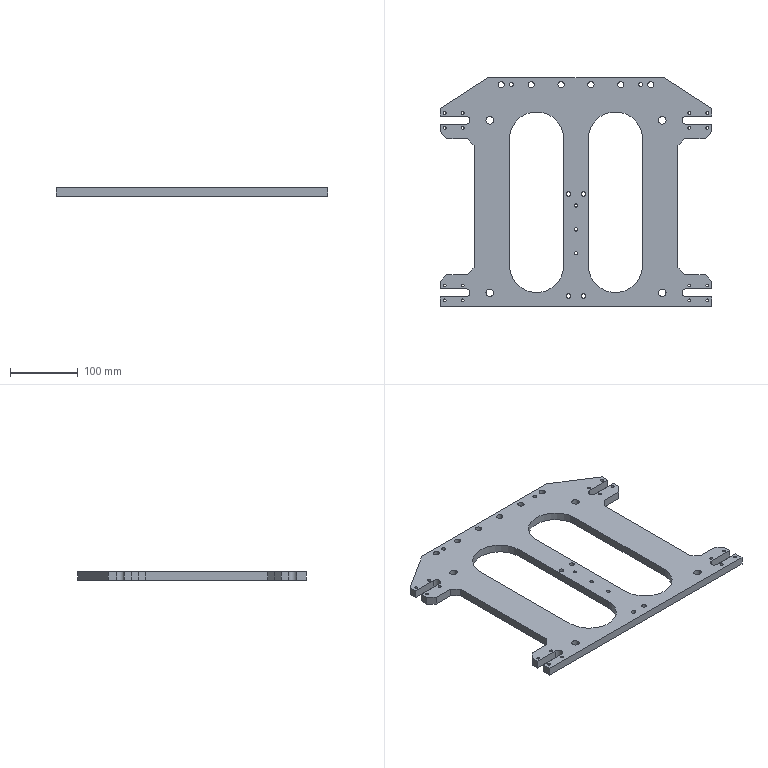NC program | NX | posted with a generic post | part box 400 x 336 x 12 mm
Lines 144 to 1129 of 3199:
(ZLEVEL_PROFILE , TOOL : D10)
N250 T10 M6
N252 G54
N254 G17 G0 G90 X-212.43 Y126.517 S2200 M3
N256 G43 Z80. H10
N258 Z2.782
N260 G94 G1 Z-0.218 F2200.
N262 X-208.293 Y124.385
N264 G3 X-207.294 Y124.433 R1.
N266 G1 X-201.168 Y128.371
N268 X-132.785 Y172.332
N270 G2 X-129.417 Y173.117 R5.15
N272 G1 X-129.365 Y173.145
N274 X-128.978
N276 X-128.93 Y173.15
N278 X130.
N280 G2 X132.785 Y172.332 R5.15
N282 G1 X201.168 Y128.371
N284 X202.314 Y127.634
N286 X202.352 Y127.582
N288 G2 X203.399 Y126.869 R5.15
N290 G1 X203.463 Y126.896
N292 X207.294 Y124.433
N294 G3 X208.293 Y124.385 R1.
N296 G1 X212.429 Y126.517
N298 Z2.782
N300 G0 Z2.564
N302 G1 Z-0.436
N304 X208.293 Y124.385
N306 G2 X207.294 Y124.433 R1.
N308 G1 X203.463 Y126.896
N310 X203.399 Y126.869
N312 G3 X202.352 Y127.582 R5.15
N314 G1 X202.314 Y127.634
N316 X201.168 Y128.371
N318 X132.785 Y172.332
N320 G3 X130. Y173.15 R5.15
N322 G1 X-128.93
N324 X-128.978 Y173.145
N326 X-129.365
N328 X-129.417 Y173.117
N330 G3 X-132.785 Y172.332 R5.15
N332 G1 X-201.168 Y128.371
N334 X-207.294 Y124.433
N336 G2 X-208.293 Y124.385 R1.
N338 G1 X-212.43 Y126.517
N340 Z2.564
N342 G0 Z2.345
N344 G1 Z-0.655
N346 X-208.293 Y124.385
N348 G3 X-207.294 Y124.433 R1.
N350 G1 X-201.168 Y128.371
N352 X-132.785 Y172.332
N354 G2 X-129.417 Y173.117 R5.15
N356 G1 X-129.365 Y173.145
N358 X-128.978
N360 X-128.93 Y173.15
N362 X130.
N364 G2 X132.785 Y172.332 R5.15
N366 G1 X201.168 Y128.371
N368 X202.314 Y127.634
N370 X202.352 Y127.582
N372 G2 X203.399 Y126.869 R5.15
N374 G1 X203.463 Y126.896
N376 X207.294 Y124.433
N378 G3 X208.293 Y124.385 R1.
N380 G1 X212.429 Y126.517
N382 Z2.345
N384 G0 Z2.127
N386 G1 Z-0.873
N388 X208.293 Y124.385
N390 G2 X207.294 Y124.433 R1.
N392 G1 X203.463 Y126.896
N394 X203.399 Y126.869
N396 G3 X202.352 Y127.582 R5.15
N398 G1 X202.314 Y127.634
N400 X201.168 Y128.371
N402 X132.785 Y172.332
N404 G3 X130. Y173.15 R5.15
N406 G1 X-128.93
N408 X-128.978 Y173.145
N410 X-129.365
N412 X-129.417 Y173.117
N414 G3 X-132.785 Y172.332 R5.15
N416 G1 X-201.168 Y128.371
N418 X-207.294 Y124.433
N420 G2 X-208.293 Y124.385 R1.
N422 G1 X-212.43 Y126.517
N424 Z2.127
N426 G0 Z1.909
N428 G1 Z-1.091
N430 X-208.293 Y124.385
N432 G3 X-207.294 Y124.433 R1.
N434 G1 X-201.168 Y128.371
N436 X-132.785 Y172.332
N438 G2 X-129.417 Y173.117 R5.15
N440 G1 X-129.365 Y173.145
N442 X-128.978
N444 X-128.93 Y173.15
N446 X130.
N448 G2 X132.785 Y172.332 R5.15
N450 G1 X201.168 Y128.371
N452 X202.314 Y127.634
N454 X202.352 Y127.582
N456 G2 X203.399 Y126.869 R5.15
N458 G1 X203.463 Y126.896
N460 X207.294 Y124.433
N462 G3 X208.293 Y124.385 R1.
N464 G1 X212.429 Y126.517
N466 Z1.909
N468 G0 Z1.691
N470 G1 Z-1.309
N472 X208.293 Y124.385
N474 G2 X207.294 Y124.433 R1.
N476 G1 X203.463 Y126.896
N478 X203.399 Y126.869
N480 G3 X202.352 Y127.582 R5.15
N482 G1 X202.314 Y127.634
N484 X201.168 Y128.371
N486 X132.785 Y172.332
N488 G3 X130. Y173.15 R5.15
N490 G1 X-128.93
N492 X-128.978 Y173.145
N494 X-129.365
N496 X-129.417 Y173.117
N498 G3 X-132.785 Y172.332 R5.15
N500 G1 X-201.168 Y128.371
N502 X-207.294 Y124.433
N504 G2 X-208.293 Y124.385 R1.
N506 G1 X-212.43 Y126.517
N508 Z1.691
N510 G0 Z1.473
N512 G1 Z-1.527
N514 X-208.293 Y124.385
N516 G3 X-207.294 Y124.433 R1.
N518 G1 X-201.168 Y128.371
N520 X-132.785 Y172.332
N522 G2 X-129.417 Y173.117 R5.15
N524 G1 X-129.365 Y173.145
N526 X-128.978
N528 X-128.93 Y173.15
N530 X130.
N532 G2 X132.785 Y172.332 R5.15
N534 G1 X201.168 Y128.371
N536 X202.314 Y127.634
N538 X202.352 Y127.582
N540 G2 X203.399 Y126.869 R5.15
N542 G1 X203.463 Y126.896
N544 X207.294 Y124.433
N546 G3 X208.293 Y124.385 R1.
N548 G1 X212.429 Y126.517
N550 Z1.473
N552 G0 Z1.255
N554 G1 Z-1.745
N556 X208.293 Y124.385
N558 G2 X207.294 Y124.433 R1.
N560 G1 X203.463 Y126.896
N562 X203.399 Y126.869
N564 G3 X202.352 Y127.582 R5.15
N566 G1 X202.314 Y127.634
N568 X201.168 Y128.371
N570 X132.785 Y172.332
N572 G3 X130. Y173.15 R5.15
N574 G1 X-128.93
N576 X-128.978 Y173.145
N578 X-129.365
N580 X-129.417 Y173.117
N582 G3 X-132.785 Y172.332 R5.15
N584 G1 X-201.168 Y128.371
N586 X-207.294 Y124.433
N588 G2 X-208.293 Y124.385 R1.
N590 G1 X-212.43 Y126.517
N592 Z1.255
N594 G0 Z1.036
N596 G1 Z-1.964
N598 X-208.293 Y124.385
N600 G3 X-207.294 Y124.433 R1.
N602 G1 X-201.168 Y128.371
N604 X-132.785 Y172.332
N606 G2 X-129.417 Y173.117 R5.15
N608 G1 X-129.365 Y173.145
N610 X-128.978
N612 X-128.93 Y173.15
N614 X130.
N616 G2 X132.785 Y172.332 R5.15
N618 G1 X201.168 Y128.371
N620 X202.314 Y127.634
N622 X202.352 Y127.582
N624 G2 X203.399 Y126.869 R5.15
N626 G1 X203.463 Y126.896
N628 X207.294 Y124.433
N630 G3 X208.293 Y124.385 R1.
N632 G1 X212.429 Y126.517
N634 Z1.036
N636 G0 Z0.818
N638 G1 Z-2.182
N640 X208.293 Y124.385
N642 G2 X207.294 Y124.433 R1.
N644 G1 X203.463 Y126.896
N646 X203.399 Y126.869
N648 G3 X202.352 Y127.582 R5.15
N650 G1 X202.314 Y127.634
N652 X201.168 Y128.371
N654 X132.785 Y172.332
N656 G3 X130. Y173.15 R5.15
N658 G1 X-128.93
N660 X-128.978 Y173.145
N662 X-129.365
N664 X-129.417 Y173.117
N666 G3 X-132.785 Y172.332 R5.15
N668 G1 X-201.168 Y128.371
N670 X-207.294 Y124.433
N672 G2 X-208.293 Y124.385 R1.
N674 G1 X-212.43 Y126.517
N676 Z0.818
N678 G0 Z0.6
N680 G1 Z-2.4
N682 X-208.293 Y124.385
N684 G3 X-207.294 Y124.433 R1.
N686 G1 X-201.168 Y128.371
N688 X-132.785 Y172.332
N690 G2 X-129.417 Y173.117 R5.15
N692 G1 X-129.365 Y173.145
N694 X-128.978
N696 X-128.93 Y173.15
N698 X130.
N700 G2 X132.785 Y172.332 R5.15
N702 G1 X201.168 Y128.371
N704 X202.314 Y127.634
N706 X202.352 Y127.582
N708 G2 X203.399 Y126.869 R5.15
N710 G1 X203.463 Y126.896
N712 X207.294 Y124.433
N714 G3 X208.293 Y124.385 R1.
N716 G1 X212.429 Y126.517
N718 Z0.6
N720 G0 Z0.382
N722 G1 Z-2.618
N724 X208.293 Y124.385
N726 G2 X207.294 Y124.433 R1.
N728 G1 X203.463 Y126.896
N730 X203.399 Y126.869
N732 G3 X202.352 Y127.582 R5.15
N734 G1 X202.314 Y127.634
N736 X201.168 Y128.371
N738 X132.785 Y172.332
N740 G3 X130. Y173.15 R5.15
N742 G1 X-128.93
N744 X-128.978 Y173.145
N746 X-129.365
N748 X-129.417 Y173.117
N750 G3 X-132.785 Y172.332 R5.15
N752 G1 X-201.168 Y128.371
N754 X-207.294 Y124.433
N756 G2 X-208.293 Y124.385 R1.
N758 G1 X-212.43 Y126.517
N760 Z0.382
N762 G0 Z0.164
N764 G1 Z-2.836
N766 X-208.293 Y124.385
N768 G3 X-207.294 Y124.433 R1.
N770 G1 X-201.168 Y128.371
N772 X-132.785 Y172.332
N774 G2 X-129.417 Y173.117 R5.15
N776 G1 X-129.365 Y173.145
N778 X-128.978
N780 X-128.93 Y173.15
N782 X130.
N784 G2 X132.785 Y172.332 R5.15
N786 G1 X201.168 Y128.371
N788 X202.314 Y127.634
N790 X202.352 Y127.582
N792 G2 X203.399 Y126.869 R5.15
N794 G1 X203.463 Y126.896
N796 X207.294 Y124.433
N798 G3 X208.293 Y124.385 R1.
N800 G1 X212.429 Y126.517
N802 Z0.164
N804 G0 Z-0.055
N806 G1 Z-3.055
N808 X208.293 Y124.385
N810 G2 X207.294 Y124.433 R1.
N812 G1 X203.463 Y126.896
N814 X203.399 Y126.869
N816 G3 X202.352 Y127.582 R5.15
N818 G1 X202.314 Y127.634
N820 X201.168 Y128.371
N822 X132.785 Y172.332
N824 G3 X130. Y173.15 R5.15
N826 G1 X-128.93
N828 X-128.978 Y173.145
N830 X-129.365
N832 X-129.417 Y173.117
N834 G3 X-132.785 Y172.332 R5.15
N836 G1 X-201.168 Y128.371
N838 X-207.294 Y124.433
N840 G2 X-208.293 Y124.385 R1.
N842 G1 X-212.43 Y126.517
N844 Z-0.055
N846 G0 Z-0.273
N848 G1 Z-3.273
N850 X-208.293 Y124.385
N852 G3 X-207.294 Y124.433 R1.
N854 G1 X-201.168 Y128.371
N856 X-132.785 Y172.332
N858 G2 X-129.417 Y173.117 R5.15
N860 G1 X-129.365 Y173.145
N862 X-128.978
N864 X-128.93 Y173.15
N866 X130.
N868 G2 X132.785 Y172.332 R5.15
N870 G1 X201.168 Y128.371
N872 X202.314 Y127.634
N874 X202.352 Y127.582
N876 G2 X203.399 Y126.869 R5.15
N878 G1 X203.463 Y126.896
N880 X207.294 Y124.433
N882 G3 X208.293 Y124.385 R1.
N884 G1 X212.429 Y126.517
N886 Z-0.273
N888 G0 Z-0.491
N890 G1 Z-3.491
N892 X208.293 Y124.385
N894 G2 X207.294 Y124.433 R1.
N896 G1 X203.463 Y126.896
N898 X203.399 Y126.869
N900 G3 X202.352 Y127.582 R5.15
N902 G1 X202.314 Y127.634
N904 X201.168 Y128.371
N906 X132.785 Y172.332
N908 G3 X130. Y173.15 R5.15
N910 G1 X-128.93
N912 X-128.978 Y173.145
N914 X-129.365
N916 X-129.417 Y173.117
N918 G3 X-132.785 Y172.332 R5.15
N920 G1 X-201.168 Y128.371
N922 X-207.294 Y124.433
N924 G2 X-208.293 Y124.385 R1.
N926 G1 X-212.43 Y126.517
N928 Z-0.491
N930 G0 Z-0.709
N932 G1 Z-3.709
N934 X-208.293 Y124.385
N936 G3 X-207.294 Y124.433 R1.
N938 G1 X-201.168 Y128.371
N940 X-132.785 Y172.332
N942 G2 X-129.417 Y173.117 R5.15
N944 G1 X-129.365 Y173.145
N946 X-128.978
N948 X-128.93 Y173.15
N950 X130.
N952 G2 X132.785 Y172.332 R5.15
N954 G1 X201.168 Y128.371
N956 X202.314 Y127.634
N958 X202.352 Y127.582
N960 G2 X203.399 Y126.869 R5.15
N962 G1 X203.463 Y126.896
N964 X207.294 Y124.433
N966 G3 X208.293 Y124.385 R1.
N968 G1 X212.429 Y126.517
N970 Z-0.709
N972 G0 Z-0.927
N974 G1 Z-3.927
N976 X208.293 Y124.385
N978 G2 X207.294 Y124.433 R1.
N980 G1 X203.463 Y126.896
N982 X203.399 Y126.869
N984 G3 X202.352 Y127.582 R5.15
N986 G1 X202.314 Y127.634
N988 X201.168 Y128.371
N990 X132.785 Y172.332
N992 G3 X130. Y173.15 R5.15
N994 G1 X-128.93
N996 X-128.978 Y173.145
N998 X-129.365
N1000 X-129.417 Y173.117
N1002 G3 X-132.785 Y172.332 R5.15
N1004 G1 X-201.168 Y128.371
N1006 X-207.294 Y124.433
N1008 G2 X-208.293 Y124.385 R1.
N1010 G1 X-212.43 Y126.517
N1012 Z-0.927
N1014 G0 Z-1.145
N1016 G1 Z-4.145
N1018 X-208.293 Y124.385
N1020 G3 X-207.294 Y124.433 R1.
N1022 G1 X-201.168 Y128.371
N1024 X-132.785 Y172.332
N1026 G2 X-129.417 Y173.117 R5.15
N1028 G1 X-129.365 Y173.145
N1030 X-128.978
N1032 X-128.93 Y173.15
N1034 X130.
N1036 G2 X132.785 Y172.332 R5.15
N1038 G1 X201.168 Y128.371
N1040 X202.314 Y127.634
N1042 X202.352 Y127.582
N1044 G2 X203.399 Y126.869 R5.15
N1046 G1 X203.463 Y126.896
N1048 X207.294 Y124.433
N1050 G3 X208.293 Y124.385 R1.
N1052 G1 X212.43 Y126.517
N1054 Z-1.145
N1056 G0 Z-1.364
N1058 G1 Z-4.364
N1060 X208.293 Y124.385
N1062 G2 X207.294 Y124.433 R1.
N1064 G1 X203.463 Y126.896
N1066 X203.399 Y126.869
N1068 G3 X202.352 Y127.582 R5.15
N1070 G1 X202.314 Y127.634
N1072 X201.168 Y128.371
N1074 X132.785 Y172.332
N1076 G3 X130. Y173.15 R5.15
N1078 G1 X-128.93
N1080 X-128.978 Y173.145
N1082 X-129.365
N1084 X-129.417 Y173.117
N1086 G3 X-132.785 Y172.332 R5.15
N1088 G1 X-201.168 Y128.371
N1090 X-207.294 Y124.433
N1092 G2 X-208.293 Y124.385 R1.
N1094 G1 X-212.43 Y126.517
N1096 Z-1.364
N1098 G0 Z-1.582
N1100 G1 Z-4.582
N1102 X-208.293 Y124.385
N1104 G3 X-207.294 Y124.433 R1.
N1106 G1 X-201.168 Y128.371
N1108 X-132.785 Y172.332
N1110 G2 X-129.417 Y173.117 R5.15
N1112 G1 X-129.365 Y173.145
N1114 X-128.978
N1116 X-128.93 Y173.15
N1118 X130.
N1120 G2 X132.785 Y172.332 R5.15
N1122 G1 X201.168 Y128.371
N1124 X202.314 Y127.634
N1126 X202.352 Y127.582
N1128 G2 X203.399 Y126.869 R5.15
N1130 G1 X203.463 Y126.896
N1132 X207.294 Y124.433
N1134 G3 X208.293 Y124.385 R1.
N1136 G1 X212.43 Y126.517
N1138 Z-1.582
N1140 G0 Z-1.8
N1142 G1 Z-4.8
N1144 X208.293 Y124.385
N1146 G2 X207.294 Y124.433 R1.
N1148 G1 X203.463 Y126.896
N1150 X203.399 Y126.869
N1152 G3 X202.352 Y127.582 R5.15
N1154 G1 X202.314 Y127.634
N1156 X201.168 Y128.371
N1158 X132.785 Y172.332
N1160 G3 X130. Y173.15 R5.15
N1162 G1 X-128.93
N1164 X-128.978 Y173.145
N1166 X-129.365
N1168 X-129.417 Y173.117
N1170 G3 X-132.785 Y172.332 R5.15
N1172 G1 X-201.168 Y128.371
N1174 X-207.294 Y124.433
N1176 G2 X-208.293 Y124.385 R1.
N1178 G1 X-212.43 Y126.517
N1180 Z-1.8
N1182 G0 Z-2.018
N1184 G1 Z-5.018
N1186 X-208.293 Y124.385
N1188 G3 X-207.294 Y124.433 R1.
N1190 G1 X-201.168 Y128.371
N1192 X-132.785 Y172.332
N1194 G2 X-129.417 Y173.117 R5.15
N1196 G1 X-129.365 Y173.145
N1198 X-128.978
N1200 X-128.93 Y173.15
N1202 X130.
N1204 G2 X132.785 Y172.332 R5.15
N1206 G1 X201.168 Y128.371
N1208 X202.314 Y127.634
N1210 X202.352 Y127.582
N1212 G2 X203.399 Y126.869 R5.15
N1214 G1 X203.463 Y126.896
N1216 X207.294 Y124.433
N1218 G3 X208.293 Y124.385 R1.
N1220 G1 X212.43 Y126.517
N1222 Z-2.018
N1224 G0 Z-2.236
N1226 G1 Z-5.236
N1228 X208.293 Y124.385
N1230 G2 X207.294 Y124.433 R1.
N1232 G1 X203.463 Y126.896
N1234 X203.399 Y126.869
N1236 G3 X202.352 Y127.582 R5.15
N1238 G1 X202.314 Y127.634
N1240 X201.168 Y128.371
N1242 X132.785 Y172.332
N1244 G3 X130. Y173.15 R5.15
N1246 G1 X-128.93
N1248 X-128.978 Y173.146
N1250 X-129.365
N1252 X-129.417 Y173.117
N1254 G3 X-132.785 Y172.332 R5.15
N1256 G1 X-201.168 Y128.371
N1258 X-207.294 Y124.433
N1260 G2 X-208.293 Y124.385 R1.
N1262 G1 X-212.43 Y126.517
N1264 Z-2.236
N1266 G0 Z-2.455
N1268 G1 Z-5.455
N1270 X-208.293 Y124.385
N1272 G3 X-207.294 Y124.433 R1.
N1274 G1 X-201.168 Y128.371
N1276 X-132.785 Y172.332
N1278 G2 X-129.417 Y173.117 R5.15
N1280 G1 X-129.365 Y173.146
N1282 X-128.978
N1284 X-128.93 Y173.15
N1286 X130.
N1288 G2 X132.785 Y172.332 R5.15
N1290 G1 X201.168 Y128.371
N1292 X202.314 Y127.634
N1294 X202.352 Y127.582
N1296 G2 X203.399 Y126.869 R5.15
N1298 G1 X203.463 Y126.896
N1300 X207.294 Y124.433
N1302 G3 X208.293 Y124.385 R1.
N1304 G1 X212.43 Y126.517
N1306 Z-2.455
N1308 G0 Z-2.673
N1310 G1 Z-5.673
N1312 X208.293 Y124.385
N1314 G2 X207.294 Y124.433 R1.
N1316 G1 X203.463 Y126.896
N1318 X203.399 Y126.869
N1320 G3 X202.352 Y127.582 R5.15
N1322 G1 X202.314 Y127.634
N1324 X201.168 Y128.371
N1326 X132.785 Y172.332
N1328 G3 X130. Y173.15 R5.15
N1330 G1 X-128.93
N1332 X-128.978 Y173.146
N1334 X-129.365
N1336 X-129.417 Y173.117
N1338 G3 X-132.785 Y172.332 R5.15
N1340 G1 X-201.168 Y128.371
N1342 X-207.294 Y124.433
N1344 G2 X-208.293 Y124.385 R1.
N1346 G1 X-212.43 Y126.517
N1348 Z-2.673
N1350 G0 Z-2.891
N1352 G1 Z-5.891
N1354 X-208.293 Y124.385
N1356 G3 X-207.294 Y124.433 R1.
N1358 G1 X-201.168 Y128.371
N1360 X-132.785 Y172.332
N1362 G2 X-129.417 Y173.117 R5.15
N1364 G1 X-129.365 Y173.146
N1366 X-128.978
N1368 X-128.93 Y173.15
N1370 X130.
N1372 G2 X132.785 Y172.332 R5.15
N1374 G1 X201.168 Y128.371
N1376 X202.314 Y127.634
N1378 X202.352 Y127.582
N1380 G2 X203.399 Y126.869 R5.15
N1382 G1 X203.463 Y126.896
N1384 X207.294 Y124.433
N1386 G3 X208.293 Y124.385 R1.
N1388 G1 X212.43 Y126.517
N1390 Z-2.891
N1392 G0 Z-3.109
N1394 G1 Z-6.109
N1396 X208.293 Y124.385
N1398 G2 X207.294 Y124.433 R1.
N1400 G1 X203.463 Y126.896
N1402 X203.399 Y126.869
N1404 G3 X202.352 Y127.582 R5.15
N1406 G1 X202.314 Y127.634
N1408 X201.168 Y128.371
N1410 X132.785 Y172.332
N1412 G3 X130. Y173.15 R5.15
N1414 G1 X-128.93
N1416 X-128.978 Y173.146
N1418 X-129.365
N1420 X-129.417 Y173.117
N1422 G3 X-132.785 Y172.332 R5.15
N1424 G1 X-201.168 Y128.371
N1426 X-207.294 Y124.433
N1428 G2 X-208.293 Y124.385 R1.
N1430 G1 X-212.43 Y126.517
N1432 Z-3.109
N1434 G0 Z-3.327
N1436 G1 Z-6.327
N1438 X-208.293 Y124.385
N1440 G3 X-207.294 Y124.433 R1.
N1442 G1 X-201.168 Y128.371
N1444 X-132.785 Y172.332
N1446 G2 X-129.417 Y173.117 R5.15
N1448 G1 X-129.365 Y173.146
N1450 X-128.978
N1452 X-128.93 Y173.15
N1454 X130.
N1456 G2 X132.785 Y172.332 R5.15
N1458 G1 X201.168 Y128.371
N1460 X202.314 Y127.634
N1462 X202.352 Y127.582
N1464 G2 X203.399 Y126.869 R5.15
N1466 G1 X203.463 Y126.896
N1468 X207.294 Y124.433
N1470 G3 X208.293 Y124.385 R1.
N1472 G1 X212.43 Y126.517
N1474 Z-3.327
N1476 G0 Z-3.545
N1478 G1 Z-6.545
N1480 X208.293 Y124.385
N1482 G2 X207.294 Y124.433 R1.
N1484 G1 X203.463 Y126.896
N1486 X203.399 Y126.869
N1488 G3 X202.352 Y127.582 R5.15
N1490 G1 X202.314 Y127.634
N1492 X201.168 Y128.371
N1494 X132.785 Y172.332
N1496 G3 X130. Y173.15 R5.15
N1498 G1 X-128.93
N1500 X-128.978 Y173.146
N1502 X-129.365
N1504 X-129.417 Y173.117
N1506 G3 X-132.785 Y172.332 R5.15
N1508 G1 X-201.168 Y128.371
N1510 X-207.294 Y124.433
N1512 G2 X-208.293 Y124.385 R1.
N1514 G1 X-212.43 Y126.517
N1516 Z-3.545
N1518 G0 Z-3.764
N1520 G1 Z-6.764
N1522 X-208.293 Y124.385
N1524 G3 X-207.294 Y124.433 R1.
N1526 G1 X-201.168 Y128.371
N1528 X-132.785 Y172.332
N1530 G2 X-129.417 Y173.117 R5.15
N1532 G1 X-129.365 Y173.146
N1534 X-128.978
N1536 X-128.93 Y173.15
N1538 X130.
N1540 G2 X132.785 Y172.332 R5.15
N1542 G1 X201.168 Y128.371
N1544 X202.314 Y127.634
N1546 X202.352 Y127.582
N1548 G2 X203.399 Y126.869 R5.15
N1550 G1 X203.463 Y126.896
N1552 X207.294 Y124.433
N1554 G3 X208.293 Y124.385 R1.
N1556 G1 X212.43 Y126.517
N1558 Z-3.764
N1560 G0 Z-3.982
N1562 G1 Z-6.982
N1564 X208.293 Y124.385
N1566 G2 X207.294 Y124.433 R1.
N1568 G1 X203.463 Y126.896
N1570 X203.399 Y126.869
N1572 G3 X202.352 Y127.582 R5.15
N1574 G1 X202.314 Y127.634
N1576 X201.168 Y128.371
N1578 X132.785 Y172.332
N1580 G3 X130. Y173.15 R5.15
N1582 G1 X-128.93
N1584 X-128.978 Y173.146
N1586 X-129.365
N1588 X-129.417 Y173.117
N1590 G3 X-132.785 Y172.332 R5.15
N1592 G1 X-201.168 Y128.371
N1594 X-207.294 Y124.433
N1596 G2 X-208.293 Y124.385 R1.
N1598 G1 X-212.43 Y126.517
N1600 Z-3.982
N1602 G0 Z-4.2
N1604 G1 Z-7.2
N1606 X-208.293 Y124.385
N1608 G3 X-207.294 Y124.433 R1.
N1610 G1 X-201.168 Y128.371
N1612 X-132.785 Y172.332
N1614 G2 X-129.417 Y173.117 R5.15
N1616 G1 X-129.365 Y173.146
N1618 X-128.978
N1620 X-128.93 Y173.15
N1622 X130.
N1624 G2 X132.785 Y172.332 R5.15
N1626 G1 X201.168 Y128.371
N1628 X202.314 Y127.634
N1630 X202.352 Y127.582
N1632 G2 X203.399 Y126.869 R5.15
N1634 G1 X203.463 Y126.896
N1636 X207.294 Y124.433
N1638 G3 X208.293 Y124.385 R1.
N1640 G1 X212.43 Y126.517
N1642 Z-4.2
N1644 G0 Z-4.418
N1646 G1 Z-7.418
N1648 X208.293 Y124.385
N1650 G2 X207.294 Y124.433 R1.
N1652 G1 X203.463 Y126.896
N1654 X203.399 Y126.869
N1656 G3 X202.352 Y127.582 R5.15
N1658 G1 X202.314 Y127.634
N1660 X201.168 Y128.371
N1662 X132.785 Y172.332
N1664 G3 X130. Y173.15 R5.15
N1666 G1 X-128.93
N1668 X-128.978 Y173.146
N1670 X-129.365
N1672 X-129.417 Y173.117
N1674 G3 X-132.785 Y172.332 R5.15
N1676 G1 X-201.168 Y128.371
N1678 X-207.294 Y124.433
N1680 G2 X-208.293 Y124.385 R1.
N1682 G1 X-212.43 Y126.517
N1684 Z-4.418
N1686 G0 Z-4.636
N1688 G1 Z-7.636
N1690 X-208.293 Y124.385
N1692 G3 X-207.294 Y124.433 R1.
N1694 G1 X-201.168 Y128.371
N1696 X-132.785 Y172.332
N1698 G2 X-129.417 Y173.117 R5.15
N1700 G1 X-129.365 Y173.146
N1702 X-128.978
N1704 X-128.93 Y173.15
N1706 X130.
N1708 G2 X132.785 Y172.332 R5.15
N1710 G1 X201.168 Y128.371
N1712 X202.314 Y127.634
N1714 X202.352 Y127.582
N1716 G2 X203.399 Y126.869 R5.15
N1718 G1 X203.463 Y126.896
N1720 X207.294 Y124.433
N1722 G3 X208.293 Y124.385 R1.
N1724 G1 X212.43 Y126.517
N1726 Z-4.636
N1728 G0 Z-4.855
N1730 G1 Z-7.855
N1732 X208.293 Y124.385
N1734 G2 X207.294 Y124.433 R1.
N1736 G1 X203.463 Y126.896
N1738 X203.399 Y126.869
N1740 G3 X202.352 Y127.582 R5.15
N1742 G1 X202.314 Y127.634
N1744 X201.168 Y128.371
N1746 X132.785 Y172.332
N1748 G3 X130. Y173.15 R5.15
N1750 G1 X-128.93
N1752 X-128.978 Y173.146
N1754 X-129.365
N1756 X-129.417 Y173.117
N1758 G3 X-132.785 Y172.332 R5.15
N1760 G1 X-201.168 Y128.371
N1762 X-207.294 Y124.433
N1764 G2 X-208.293 Y124.385 R1.
N1766 G1 X-212.43 Y126.517
N1768 Z-4.855
N1770 G0 Z-5.073
N1772 G1 Z-8.073
N1774 X-208.293 Y124.385
N1776 G3 X-207.294 Y124.433 R1.
N1778 G1 X-201.168 Y128.371
N1780 X-132.785 Y172.332
N1782 G2 X-129.417 Y173.117 R5.15
N1784 G1 X-129.365 Y173.146
N1786 X-128.978
N1788 X-128.93 Y173.15
N1790 X130.
N1792 G2 X132.785 Y172.332 R5.15
N1794 G1 X201.168 Y128.371
N1796 X202.314 Y127.634
N1798 X202.352 Y127.582
N1800 G2 X203.399 Y126.869 R5.15
N1802 G1 X203.463 Y126.896
N1804 X207.294 Y124.433
N1806 G3 X208.293 Y124.385 R1.
N1808 G1 X212.43 Y126.517
N1810 Z-5.073
N1812 G0 Z-5.291
N1814 G1 Z-8.291
N1816 X208.293 Y124.385
N1818 G2 X207.294 Y124.433 R1.
N1820 G1 X203.463 Y126.896
N1822 X203.399 Y126.869
N1824 G3 X202.352 Y127.582 R5.15
N1826 G1 X202.314 Y127.634
N1828 X201.168 Y128.371
N1830 X132.785 Y172.332
N1832 G3 X130. Y173.15 R5.15
N1834 G1 X-128.93
N1836 X-128.978 Y173.146
N1838 X-129.365
N1840 X-129.417 Y173.117
N1842 G3 X-132.785 Y172.332 R5.15
N1844 G1 X-201.168 Y128.371
N1846 X-207.294 Y124.433
N1848 G2 X-208.293 Y124.385 R1.
N1850 G1 X-212.43 Y126.517
N1852 Z-5.291
N1854 G0 Z-5.509
N1856 G1 Z-8.509
N1858 X-208.293 Y124.385
N1860 G3 X-207.294 Y124.433 R1.
N1862 G1 X-201.168 Y128.371
N1864 X-132.785 Y172.332
N1866 G2 X-129.417 Y173.117 R5.15
N1868 G1 X-129.365 Y173.146
N1870 X-128.978
N1872 X-128.93 Y173.15
N1874 X130.
N1876 G2 X132.785 Y172.332 R5.15
N1878 G1 X201.168 Y128.371
N1880 X202.314 Y127.634
N1882 X202.352 Y127.582
N1884 G2 X203.399 Y126.869 R5.15
N1886 G1 X203.463 Y126.896
N1888 X207.294 Y124.433
N1890 G3 X208.293 Y124.385 R1.
N1892 G1 X212.43 Y126.517
N1894 Z-5.509
N1896 G0 Y126.518 Z-5.727
N1898 G1 Z-8.727
N1900 X208.293 Y124.385
N1902 G2 X207.294 Y124.433 R1.
N1904 G1 X203.463 Y126.896
N1906 X203.399 Y126.869
N1908 G3 X202.352 Y127.582 R5.15
N1910 G1 X202.314 Y127.634
N1912 X201.168 Y128.371
N1914 X132.785 Y172.332
N1916 G3 X130. Y173.15 R5.15
N1918 G1 X-128.93
N1920 X-128.978 Y173.146
N1922 X-129.365
N1924 X-129.417 Y173.117
N1926 G3 X-132.785 Y172.332 R5.15
N1928 G1 X-201.168 Y128.371
N1930 X-207.294 Y124.433
N1932 G2 X-208.293 Y124.385 R1.
N1934 G1 X-212.43 Y126.517
N1936 Z-5.727
N1938 G0 Z-5.945
N1940 G1 Z-8.945
N1942 X-208.293 Y124.385
N1944 G3 X-207.294 Y124.433 R1.
N1946 G1 X-201.168 Y128.371
N1948 X-132.785 Y172.332
N1950 G2 X-129.417 Y173.117 R5.15
N1952 G1 X-129.365 Y173.146
N1954 X-128.978
N1956 X-128.93 Y173.15
N1958 X130.
N1960 G2 X132.785 Y172.332 R5.15
N1962 G1 X201.168 Y128.371
N1964 X202.314 Y127.634
N1966 X202.352 Y127.582
N1968 G2 X203.399 Y126.869 R5.15
N1970 G1 X203.463 Y126.896
N1972 X207.294 Y124.433
N1974 G3 X208.293 Y124.385 R1.
N1976 G1 X212.43 Y126.518
N1978 Z-5.945
N1980 G0 Z-6.164
N1982 G1 Z-9.164
N1984 X208.293 Y124.385
N1986 G2 X207.294 Y124.433 R1.
N1988 G1 X203.463 Y126.896
N1990 X203.399 Y126.869
N1992 G3 X202.352 Y127.582 R5.15
N1994 G1 X202.314 Y127.634
N1996 X201.168 Y128.371
N1998 X132.785 Y172.332
N2000 G3 X130. Y173.15 R5.15
N2002 G1 X-128.93
N2004 X-128.978 Y173.146
N2006 X-129.365
N2008 X-129.417 Y173.117
N2010 G3 X-132.785 Y172.332 R5.15
N2012 G1 X-201.168 Y128.371
N2014 X-207.294 Y124.433
N2016 G2 X-208.293 Y124.385 R1.
N2018 G1 X-212.43 Y126.517
N2020 Z-6.164
N2022 G0 Z-6.382
N2024 G1 Z-9.382
N2026 X-208.293 Y124.385
N2028 G3 X-207.294 Y124.433 R1.
N2030 G1 X-201.168 Y128.371
N2032 X-132.785 Y172.332
N2034 G2 X-129.417 Y173.117 R5.15
N2036 G1 X-129.365 Y173.146
N2038 X-128.978
N2040 X-128.93 Y173.15
N2042 X130.
N2044 G2 X132.785 Y172.332 R5.15
N2046 G1 X201.168 Y128.371
N2048 X202.314 Y127.634
N2050 X202.352 Y127.582
N2052 G2 X203.399 Y126.869 R5.15
N2054 G1 X203.463 Y126.896
N2056 X207.294 Y124.433
N2058 G3 X208.293 Y124.385 R1.
N2060 G1 X212.43 Y126.518
N2062 Z-6.382
N2064 G0 Z-6.6
N2066 G1 Z-9.6
N2068 X208.293 Y124.385
N2070 G2 X207.294 Y124.433 R1.
N2072 G1 X203.463 Y126.896
N2074 X203.399 Y126.869
N2076 G3 X202.352 Y127.582 R5.15
N2078 G1 X202.314 Y127.634
N2080 X201.168 Y128.371
N2082 X132.785 Y172.332
N2084 G3 X130. Y173.15 R5.15
N2086 G1 X-128.93
N2088 X-128.978 Y173.146
N2090 X-129.365
N2092 X-129.417 Y173.117
N2094 G3 X-132.785 Y172.332 R5.15
N2096 G1 X-201.168 Y128.371
N2098 X-207.294 Y124.433
N2100 G2 X-208.293 Y124.385 R1.
N2102 G1 X-212.43 Y126.517
N2104 Z-6.6
N2106 G0 Z-6.818
N2108 G1 Z-9.818
N2110 X-208.293 Y124.385
N2112 G3 X-207.294 Y124.433 R1.
N2114 G1 X-201.168 Y128.371
N2116 X-132.785 Y172.332
N2118 G2 X-129.417 Y173.117 R5.15
N2120 G1 X-129.365 Y173.146
N2122 X-128.978
N2124 X-128.93 Y173.15
N2126 X130.
N2128 G2 X132.785 Y172.332 R5.15
N2130 G1 X201.168 Y128.371
N2132 X202.314 Y127.634
N2134 X202.352 Y127.582
N2136 G2 X203.399 Y126.869 R5.15
N2138 G1 X203.463 Y126.896
N2140 X207.294 Y124.433
N2142 G3 X208.293 Y124.385 R1.
N2144 G1 X212.43 Y126.518
N2146 Z-6.818
N2148 G0 Z-7.036
N2150 G1 Z-10.036
N2152 X208.293 Y124.385
N2154 G2 X207.294 Y124.433 R1.
N2156 G1 X203.463 Y126.896
N2158 X203.399 Y126.869
N2160 G3 X202.352 Y127.582 R5.15
N2162 G1 X202.314 Y127.634
N2164 X201.168 Y128.371
N2166 X132.785 Y172.332
N2168 G3 X130. Y173.15 R5.15
N2170 G1 X-128.93
N2172 X-128.978 Y173.146
N2174 X-129.365
N2176 X-129.417 Y173.117
N2178 G3 X-132.785 Y172.332 R5.15
N2180 G1 X-201.168 Y128.371
N2182 X-207.294 Y124.433
N2184 G2 X-208.293 Y124.385 R1.
N2186 G1 X-212.43 Y126.517
N2188 Z-7.036
N2190 G0 Z-7.255
N2192 G1 Z-10.255
N2194 X-208.293 Y124.385
N2196 G3 X-207.294 Y124.433 R1.
N2198 G1 X-201.168 Y128.371
N2200 X-132.785 Y172.332
N2202 G2 X-129.417 Y173.117 R5.15
N2204 G1 X-129.365 Y173.146
N2206 X-128.978
N2208 X-128.93 Y173.15
N2210 X130.
N2212 G2 X132.785 Y172.332 R5.15
N2214 G1 X201.168 Y128.371